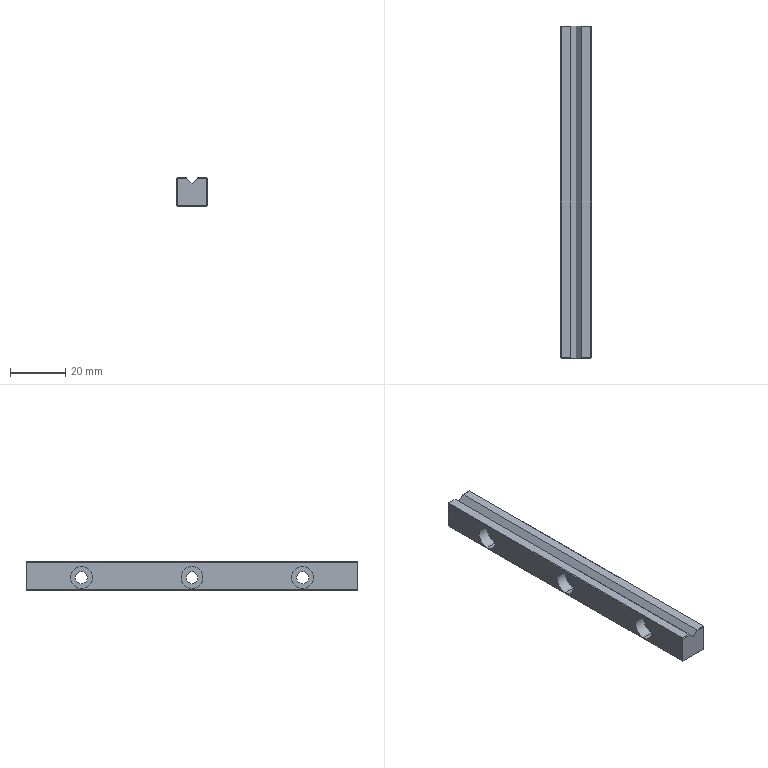Part | STEP file | 1 solid | 38 faces | box 11 x 120 x 10.2 mm | volume 12030 mm3 | plane 26 | cylinder 12 | commonest cylinder face diameters 4.3 x6 8 x6
STEP:
#1=CARTESIAN_POINT('',(-12.5,22.5,-37.85));
#2=VERTEX_POINT('',#1);
#3=CARTESIAN_POINT('',(-12.5,22.5,-42.15));
#4=VERTEX_POINT('',#3);
#5=CARTESIAN_POINT('',(-12.5,22.5,-40.));
#6=DIRECTION('',(1.,0.,0.));
#7=DIRECTION('',(0.,0.,1.));
#8=AXIS2_PLACEMENT_3D('',#5,#6,#7);
#9=CIRCLE('',#8,2.15);
#10=EDGE_CURVE('',#2,#4,#9,.T.);
#11=ORIENTED_EDGE('',*,*,#10,.T.);
#12=CARTESIAN_POINT('',(-19.3,22.5,-42.15));
#13=VERTEX_POINT('',#12);
#14=CARTESIAN_POINT('',(-12.5,22.5,-42.15));
#15=DIRECTION('',(-1.,0.,0.));
#16=VECTOR('',#15,1000.);
#17=LINE('',#14,#16);
#18=EDGE_CURVE('',#4,#13,#17,.T.);
#19=ORIENTED_EDGE('',*,*,#18,.T.);
#20=CARTESIAN_POINT('',(-19.3,22.5,-37.85));
#21=VERTEX_POINT('',#20);
#22=CARTESIAN_POINT('',(-19.3,22.5,-40.));
#23=DIRECTION('',(1.,0.,0.));
#24=DIRECTION('',(0.,0.,1.));
#25=AXIS2_PLACEMENT_3D('',#22,#23,#24);
#26=CIRCLE('',#25,2.15);
#27=EDGE_CURVE('',#21,#13,#26,.T.);
#28=ORIENTED_EDGE('',*,*,#27,.F.);
#29=CARTESIAN_POINT('',(-12.5,22.5,-37.85));
#30=DIRECTION('',(-1.,0.,0.));
#31=VECTOR('',#30,1000.);
#32=LINE('',#29,#31);
#33=EDGE_CURVE('',#2,#21,#32,.T.);
#34=ORIENTED_EDGE('',*,*,#33,.F.);
#35=EDGE_LOOP('',(#11,#19,#28,#34));
#36=FACE_OUTER_BOUND('',#35,.T.);
#37=CARTESIAN_POINT('',(-12.5,22.5,-40.));
#38=DIRECTION('',(-1.,0.,0.));
#39=DIRECTION('',(0.,0.,1.));
#40=AXIS2_PLACEMENT_3D('',#37,#38,#39);
#41=CYLINDRICAL_SURFACE('',#40,2.15);
#42=ADVANCED_FACE('',(#36),#41,.F.);
#43=CARTESIAN_POINT('',(-12.5,-17.5,-37.85));
#44=VERTEX_POINT('',#43);
#45=CARTESIAN_POINT('',(-12.5,-17.5,-42.15));
#46=VERTEX_POINT('',#45);
#47=CARTESIAN_POINT('',(-12.5,-17.5,-40.));
#48=DIRECTION('',(1.,0.,0.));
#49=DIRECTION('',(0.,0.,1.));
#50=AXIS2_PLACEMENT_3D('',#47,#48,#49);
#51=CIRCLE('',#50,2.15);
#52=EDGE_CURVE('',#44,#46,#51,.T.);
#53=ORIENTED_EDGE('',*,*,#52,.T.);
#54=CARTESIAN_POINT('',(-19.3,-17.5,-42.15));
#55=VERTEX_POINT('',#54);
#56=CARTESIAN_POINT('',(-12.5,-17.5,-42.15));
#57=DIRECTION('',(-1.,0.,0.));
#58=VECTOR('',#57,1000.);
#59=LINE('',#56,#58);
#60=EDGE_CURVE('',#46,#55,#59,.T.);
#61=ORIENTED_EDGE('',*,*,#60,.T.);
#62=CARTESIAN_POINT('',(-19.3,-17.5,-37.85));
#63=VERTEX_POINT('',#62);
#64=CARTESIAN_POINT('',(-19.3,-17.5,-40.));
#65=DIRECTION('',(1.,0.,0.));
#66=DIRECTION('',(0.,0.,1.));
#67=AXIS2_PLACEMENT_3D('',#64,#65,#66);
#68=CIRCLE('',#67,2.15);
#69=EDGE_CURVE('',#63,#55,#68,.T.);
#70=ORIENTED_EDGE('',*,*,#69,.F.);
#71=CARTESIAN_POINT('',(-12.5,-17.5,-37.85));
#72=DIRECTION('',(-1.,0.,0.));
#73=VECTOR('',#72,1000.);
#74=LINE('',#71,#73);
#75=EDGE_CURVE('',#44,#63,#74,.T.);
#76=ORIENTED_EDGE('',*,*,#75,.F.);
#77=EDGE_LOOP('',(#53,#61,#70,#76));
#78=FACE_OUTER_BOUND('',#77,.T.);
#79=CARTESIAN_POINT('',(-12.5,-17.5,-40.));
#80=DIRECTION('',(-1.,0.,0.));
#81=DIRECTION('',(0.,0.,1.));
#82=AXIS2_PLACEMENT_3D('',#79,#80,#81);
#83=CYLINDRICAL_SURFACE('',#82,2.15);
#84=ADVANCED_FACE('',(#78),#83,.F.);
#85=CARTESIAN_POINT('',(-12.5,-57.5,-37.85));
#86=VERTEX_POINT('',#85);
#87=CARTESIAN_POINT('',(-12.5,-57.5,-42.15));
#88=VERTEX_POINT('',#87);
#89=CARTESIAN_POINT('',(-12.5,-57.5,-40.));
#90=DIRECTION('',(1.,0.,0.));
#91=DIRECTION('',(0.,0.,1.));
#92=AXIS2_PLACEMENT_3D('',#89,#90,#91);
#93=CIRCLE('',#92,2.15);
#94=EDGE_CURVE('',#86,#88,#93,.T.);
#95=ORIENTED_EDGE('',*,*,#94,.T.);
#96=CARTESIAN_POINT('',(-19.3,-57.5,-42.15));
#97=VERTEX_POINT('',#96);
#98=CARTESIAN_POINT('',(-12.5,-57.5,-42.15));
#99=DIRECTION('',(-1.,0.,0.));
#100=VECTOR('',#99,1000.);
#101=LINE('',#98,#100);
#102=EDGE_CURVE('',#88,#97,#101,.T.);
#103=ORIENTED_EDGE('',*,*,#102,.T.);
#104=CARTESIAN_POINT('',(-19.3,-57.5,-37.85));
#105=VERTEX_POINT('',#104);
#106=CARTESIAN_POINT('',(-19.3,-57.5,-40.));
#107=DIRECTION('',(1.,0.,0.));
#108=DIRECTION('',(0.,0.,1.));
#109=AXIS2_PLACEMENT_3D('',#106,#107,#108);
#110=CIRCLE('',#109,2.15);
#111=EDGE_CURVE('',#105,#97,#110,.T.);
#112=ORIENTED_EDGE('',*,*,#111,.F.);
#113=CARTESIAN_POINT('',(-12.5,-57.5,-37.85));
#114=DIRECTION('',(-1.,0.,0.));
#115=VECTOR('',#114,1000.);
#116=LINE('',#113,#115);
#117=EDGE_CURVE('',#86,#105,#116,.T.);
#118=ORIENTED_EDGE('',*,*,#117,.F.);
#119=EDGE_LOOP('',(#95,#103,#112,#118));
#120=FACE_OUTER_BOUND('',#119,.T.);
#121=CARTESIAN_POINT('',(-12.5,-57.5,-40.));
#122=DIRECTION('',(-1.,0.,0.));
#123=DIRECTION('',(0.,0.,1.));
#124=AXIS2_PLACEMENT_3D('',#121,#122,#123);
#125=CYLINDRICAL_SURFACE('',#124,2.15);
#126=ADVANCED_FACE('',(#120),#125,.F.);
#127=CARTESIAN_POINT('',(-19.3,22.5,-44.));
#128=VERTEX_POINT('',#127);
#129=CARTESIAN_POINT('',(-19.3,22.5,-36.));
#130=VERTEX_POINT('',#129);
#131=CARTESIAN_POINT('',(-19.3,22.5,-40.));
#132=DIRECTION('',(-1.,0.,0.));
#133=DIRECTION('',(0.,0.,1.));
#134=AXIS2_PLACEMENT_3D('',#131,#132,#133);
#135=CIRCLE('',#134,4.);
#136=EDGE_CURVE('',#128,#130,#135,.T.);
#137=ORIENTED_EDGE('',*,*,#136,.F.);
#138=CARTESIAN_POINT('',(-23.5,22.5,-44.));
#139=VERTEX_POINT('',#138);
#140=CARTESIAN_POINT('',(-19.3,22.5,-44.));
#141=DIRECTION('',(-1.,0.,0.));
#142=VECTOR('',#141,1000.);
#143=LINE('',#140,#142);
#144=EDGE_CURVE('',#128,#139,#143,.T.);
#145=ORIENTED_EDGE('',*,*,#144,.T.);
#146=CARTESIAN_POINT('',(-23.5,22.5,-36.));
#147=VERTEX_POINT('',#146);
#148=CARTESIAN_POINT('',(-23.5,22.5,-40.));
#149=DIRECTION('',(-1.,0.,0.));
#150=DIRECTION('',(0.,0.,1.));
#151=AXIS2_PLACEMENT_3D('',#148,#149,#150);
#152=CIRCLE('',#151,4.);
#153=EDGE_CURVE('',#139,#147,#152,.T.);
#154=ORIENTED_EDGE('',*,*,#153,.T.);
#155=CARTESIAN_POINT('',(-19.3,22.5,-36.));
#156=DIRECTION('',(-1.,0.,0.));
#157=VECTOR('',#156,1000.);
#158=LINE('',#155,#157);
#159=EDGE_CURVE('',#130,#147,#158,.T.);
#160=ORIENTED_EDGE('',*,*,#159,.F.);
#161=EDGE_LOOP('',(#137,#145,#154,#160));
#162=FACE_OUTER_BOUND('',#161,.T.);
#163=CARTESIAN_POINT('',(-19.3,22.5,-40.));
#164=DIRECTION('',(-1.,0.,0.));
#165=DIRECTION('',(0.,0.,1.));
#166=AXIS2_PLACEMENT_3D('',#163,#164,#165);
#167=CYLINDRICAL_SURFACE('',#166,4.);
#168=ADVANCED_FACE('',(#162),#167,.F.);
#169=CARTESIAN_POINT('',(-19.3,-17.5,-44.));
#170=VERTEX_POINT('',#169);
#171=CARTESIAN_POINT('',(-19.3,-17.5,-36.));
#172=VERTEX_POINT('',#171);
#173=CARTESIAN_POINT('',(-19.3,-17.5,-40.));
#174=DIRECTION('',(-1.,0.,0.));
#175=DIRECTION('',(0.,0.,1.));
#176=AXIS2_PLACEMENT_3D('',#173,#174,#175);
#177=CIRCLE('',#176,4.);
#178=EDGE_CURVE('',#170,#172,#177,.T.);
#179=ORIENTED_EDGE('',*,*,#178,.F.);
#180=CARTESIAN_POINT('',(-23.5,-17.5,-44.));
#181=VERTEX_POINT('',#180);
#182=CARTESIAN_POINT('',(-19.3,-17.5,-44.));
#183=DIRECTION('',(-1.,0.,0.));
#184=VECTOR('',#183,1000.);
#185=LINE('',#182,#184);
#186=EDGE_CURVE('',#170,#181,#185,.T.);
#187=ORIENTED_EDGE('',*,*,#186,.T.);
#188=CARTESIAN_POINT('',(-23.5,-17.5,-36.));
#189=VERTEX_POINT('',#188);
#190=CARTESIAN_POINT('',(-23.5,-17.5,-40.));
#191=DIRECTION('',(-1.,0.,0.));
#192=DIRECTION('',(0.,0.,1.));
#193=AXIS2_PLACEMENT_3D('',#190,#191,#192);
#194=CIRCLE('',#193,4.);
#195=EDGE_CURVE('',#181,#189,#194,.T.);
#196=ORIENTED_EDGE('',*,*,#195,.T.);
#197=CARTESIAN_POINT('',(-19.3,-17.5,-36.));
#198=DIRECTION('',(-1.,0.,0.));
#199=VECTOR('',#198,1000.);
#200=LINE('',#197,#199);
#201=EDGE_CURVE('',#172,#189,#200,.T.);
#202=ORIENTED_EDGE('',*,*,#201,.F.);
#203=EDGE_LOOP('',(#179,#187,#196,#202));
#204=FACE_OUTER_BOUND('',#203,.T.);
#205=CARTESIAN_POINT('',(-19.3,-17.5,-40.));
#206=DIRECTION('',(-1.,0.,0.));
#207=DIRECTION('',(0.,0.,1.));
#208=AXIS2_PLACEMENT_3D('',#205,#206,#207);
#209=CYLINDRICAL_SURFACE('',#208,4.);
#210=ADVANCED_FACE('',(#204),#209,.F.);
#211=CARTESIAN_POINT('',(-19.3,-57.5,-44.));
#212=VERTEX_POINT('',#211);
#213=CARTESIAN_POINT('',(-19.3,-57.5,-36.));
#214=VERTEX_POINT('',#213);
#215=CARTESIAN_POINT('',(-19.3,-57.5,-40.));
#216=DIRECTION('',(-1.,0.,0.));
#217=DIRECTION('',(0.,0.,1.));
#218=AXIS2_PLACEMENT_3D('',#215,#216,#217);
#219=CIRCLE('',#218,4.);
#220=EDGE_CURVE('',#212,#214,#219,.T.);
#221=ORIENTED_EDGE('',*,*,#220,.F.);
#222=CARTESIAN_POINT('',(-23.5,-57.5,-44.));
#223=VERTEX_POINT('',#222);
#224=CARTESIAN_POINT('',(-19.3,-57.5,-44.));
#225=DIRECTION('',(-1.,0.,0.));
#226=VECTOR('',#225,1000.);
#227=LINE('',#224,#226);
#228=EDGE_CURVE('',#212,#223,#227,.T.);
#229=ORIENTED_EDGE('',*,*,#228,.T.);
#230=CARTESIAN_POINT('',(-23.5,-57.5,-36.));
#231=VERTEX_POINT('',#230);
#232=CARTESIAN_POINT('',(-23.5,-57.5,-40.));
#233=DIRECTION('',(-1.,0.,0.));
#234=DIRECTION('',(0.,0.,1.));
#235=AXIS2_PLACEMENT_3D('',#232,#233,#234);
#236=CIRCLE('',#235,4.);
#237=EDGE_CURVE('',#223,#231,#236,.T.);
#238=ORIENTED_EDGE('',*,*,#237,.T.);
#239=CARTESIAN_POINT('',(-19.3,-57.5,-36.));
#240=DIRECTION('',(-1.,0.,0.));
#241=VECTOR('',#240,1000.);
#242=LINE('',#239,#241);
#243=EDGE_CURVE('',#214,#231,#242,.T.);
#244=ORIENTED_EDGE('',*,*,#243,.F.);
#245=EDGE_LOOP('',(#221,#229,#238,#244));
#246=FACE_OUTER_BOUND('',#245,.T.);
#247=CARTESIAN_POINT('',(-19.3,-57.5,-40.));
#248=DIRECTION('',(-1.,0.,0.));
#249=DIRECTION('',(0.,0.,1.));
#250=AXIS2_PLACEMENT_3D('',#247,#248,#249);
#251=CYLINDRICAL_SURFACE('',#250,4.);
#252=ADVANCED_FACE('',(#246),#251,.F.);
#253=CARTESIAN_POINT('',(-16.172,42.5,-34.5));
#254=VERTEX_POINT('',#253);
#255=CARTESIAN_POINT('',(-18.,42.5,-36.328));
#256=VERTEX_POINT('',#255);
#257=CARTESIAN_POINT('',(-18.103,42.5,-36.431));
#258=DIRECTION('',(-0.7071,0.,-0.7071));
#259=VECTOR('',#258,1000.);
#260=LINE('',#257,#259);
#261=EDGE_CURVE('',#254,#256,#260,.T.);
#262=ORIENTED_EDGE('',*,*,#261,.F.);
#263=CARTESIAN_POINT('',(-12.7,42.5,-34.5));
#264=VERTEX_POINT('',#263);
#265=CARTESIAN_POINT('',(-18.,42.5,-34.5));
#266=DIRECTION('',(-1.,0.,0.));
#267=VECTOR('',#266,1000.);
#268=LINE('',#265,#267);
#269=EDGE_CURVE('',#264,#254,#268,.T.);
#270=ORIENTED_EDGE('',*,*,#269,.F.);
#271=CARTESIAN_POINT('',(-12.7,42.5,-44.3));
#272=VERTEX_POINT('',#271);
#273=CARTESIAN_POINT('',(-12.7,42.5,-39.4));
#274=DIRECTION('',(0.,0.,1.));
#275=VECTOR('',#274,1000.);
#276=LINE('',#273,#275);
#277=EDGE_CURVE('',#272,#264,#276,.T.);
#278=ORIENTED_EDGE('',*,*,#277,.F.);
#279=CARTESIAN_POINT('',(-23.3,42.5,-44.3));
#280=VERTEX_POINT('',#279);
#281=CARTESIAN_POINT('',(-18.,42.5,-44.3));
#282=DIRECTION('',(1.,0.,0.));
#283=VECTOR('',#282,1000.);
#284=LINE('',#281,#283);
#285=EDGE_CURVE('',#280,#272,#284,.T.);
#286=ORIENTED_EDGE('',*,*,#285,.F.);
#287=CARTESIAN_POINT('',(-23.3,42.5,-34.5));
#288=VERTEX_POINT('',#287);
#289=CARTESIAN_POINT('',(-23.3,42.5,-39.4));
#290=DIRECTION('',(0.,0.,-1.));
#291=VECTOR('',#290,1000.);
#292=LINE('',#289,#291);
#293=EDGE_CURVE('',#288,#280,#292,.T.);
#294=ORIENTED_EDGE('',*,*,#293,.F.);
#295=CARTESIAN_POINT('',(-19.828,42.5,-34.5));
#296=VERTEX_POINT('',#295);
#297=CARTESIAN_POINT('',(-18.,42.5,-34.5));
#298=DIRECTION('',(-1.,0.,0.));
#299=VECTOR('',#298,1000.);
#300=LINE('',#297,#299);
#301=EDGE_CURVE('',#296,#288,#300,.T.);
#302=ORIENTED_EDGE('',*,*,#301,.F.);
#303=CARTESIAN_POINT('',(-20.131,42.5,-34.197));
#304=DIRECTION('',(-0.7071,0.,0.7071));
#305=VECTOR('',#304,1000.);
#306=LINE('',#303,#305);
#307=EDGE_CURVE('',#256,#296,#306,.T.);
#308=ORIENTED_EDGE('',*,*,#307,.F.);
#309=EDGE_LOOP('',(#262,#270,#278,#286,#294,#302,#308));
#310=FACE_OUTER_BOUND('',#309,.T.);
#311=CARTESIAN_POINT('',(-12.488,42.5,-34.304));
#312=DIRECTION('',(0.,-1.,0.));
#313=DIRECTION('',(-1.,0.,0.));
#314=AXIS2_PLACEMENT_3D('',#311,#312,#313);
#315=PLANE('',#314);
#316=ADVANCED_FACE('',(#310),#315,.F.);
#317=CARTESIAN_POINT('',(-18.,-77.5,-36.328));
#318=VERTEX_POINT('',#317);
#319=CARTESIAN_POINT('',(-18.,-17.5,-36.328));
#320=DIRECTION('',(0.,-1.,0.));
#321=VECTOR('',#320,1000.);
#322=LINE('',#319,#321);
#323=EDGE_CURVE('',#256,#318,#322,.T.);
#324=ORIENTED_EDGE('',*,*,#323,.F.);
#325=ORIENTED_EDGE('',*,*,#307,.T.);
#326=CARTESIAN_POINT('',(-20.028,42.3,-34.3));
#327=VERTEX_POINT('',#326);
#328=CARTESIAN_POINT('',(-20.028,42.3,-34.3));
#329=DIRECTION('',(0.5774,0.5774,-0.5774));
#330=VECTOR('',#329,1000.);
#331=LINE('',#328,#330);
#332=EDGE_CURVE('',#327,#296,#331,.T.);
#333=ORIENTED_EDGE('',*,*,#332,.F.);
#334=CARTESIAN_POINT('',(-20.028,-77.3,-34.3));
#335=VERTEX_POINT('',#334);
#336=CARTESIAN_POINT('',(-20.028,-17.5,-34.3));
#337=DIRECTION('',(0.,1.,0.));
#338=VECTOR('',#337,1000.);
#339=LINE('',#336,#338);
#340=EDGE_CURVE('',#335,#327,#339,.T.);
#341=ORIENTED_EDGE('',*,*,#340,.F.);
#342=CARTESIAN_POINT('',(-19.828,-77.5,-34.5));
#343=VERTEX_POINT('',#342);
#344=CARTESIAN_POINT('',(-20.028,-77.3,-34.3));
#345=DIRECTION('',(0.5774,-0.5774,-0.5774));
#346=VECTOR('',#345,1000.);
#347=LINE('',#344,#346);
#348=EDGE_CURVE('',#335,#343,#347,.T.);
#349=ORIENTED_EDGE('',*,*,#348,.T.);
#350=CARTESIAN_POINT('',(-19.014,-77.5,-35.314));
#351=DIRECTION('',(-0.7071,0.,0.7071));
#352=VECTOR('',#351,1000.);
#353=LINE('',#350,#352);
#354=EDGE_CURVE('',#318,#343,#353,.T.);
#355=ORIENTED_EDGE('',*,*,#354,.F.);
#356=EDGE_LOOP('',(#324,#325,#333,#341,#349,#355));
#357=FACE_OUTER_BOUND('',#356,.T.);
#358=CARTESIAN_POINT('',(-20.131,44.9,-34.197));
#359=DIRECTION('',(-0.7071,0.,-0.7071));
#360=DIRECTION('',(0.7071,0.,-0.7071));
#361=AXIS2_PLACEMENT_3D('',#358,#359,#360);
#362=PLANE('',#361);
#363=ADVANCED_FACE('',(#357),#362,.F.);
#364=CARTESIAN_POINT('',(-15.972,42.3,-34.3));
#365=VERTEX_POINT('',#364);
#366=CARTESIAN_POINT('',(-16.172,42.5,-34.5));
#367=DIRECTION('',(0.5774,-0.5774,0.5774));
#368=VECTOR('',#367,1000.);
#369=LINE('',#366,#368);
#370=EDGE_CURVE('',#254,#365,#369,.T.);
#371=ORIENTED_EDGE('',*,*,#370,.F.);
#372=ORIENTED_EDGE('',*,*,#261,.T.);
#373=ORIENTED_EDGE('',*,*,#323,.T.);
#374=CARTESIAN_POINT('',(-16.172,-77.5,-34.5));
#375=VERTEX_POINT('',#374);
#376=CARTESIAN_POINT('',(-16.986,-77.5,-35.314));
#377=DIRECTION('',(-0.7071,0.,-0.7071));
#378=VECTOR('',#377,1000.);
#379=LINE('',#376,#378);
#380=EDGE_CURVE('',#375,#318,#379,.T.);
#381=ORIENTED_EDGE('',*,*,#380,.F.);
#382=CARTESIAN_POINT('',(-15.972,-77.3,-34.3));
#383=VERTEX_POINT('',#382);
#384=CARTESIAN_POINT('',(-16.172,-77.5,-34.5));
#385=DIRECTION('',(0.5774,0.5774,0.5774));
#386=VECTOR('',#385,1000.);
#387=LINE('',#384,#386);
#388=EDGE_CURVE('',#375,#383,#387,.T.);
#389=ORIENTED_EDGE('',*,*,#388,.T.);
#390=CARTESIAN_POINT('',(-15.972,-17.5,-34.3));
#391=DIRECTION('',(0.,-1.,0.));
#392=VECTOR('',#391,1000.);
#393=LINE('',#390,#392);
#394=EDGE_CURVE('',#365,#383,#393,.T.);
#395=ORIENTED_EDGE('',*,*,#394,.F.);
#396=EDGE_LOOP('',(#371,#372,#373,#381,#389,#395));
#397=FACE_OUTER_BOUND('',#396,.T.);
#398=CARTESIAN_POINT('',(-18.103,44.9,-36.431));
#399=DIRECTION('',(0.7071,0.,-0.7071));
#400=DIRECTION('',(0.7071,0.,0.7071));
#401=AXIS2_PLACEMENT_3D('',#398,#399,#400);
#402=PLANE('',#401);
#403=ADVANCED_FACE('',(#397),#402,.F.);
#404=CARTESIAN_POINT('',(-12.7,42.3,-34.3));
#405=VERTEX_POINT('',#404);
#406=CARTESIAN_POINT('',(-12.6,42.4,-34.4));
#407=VERTEX_POINT('',#406);
#408=CARTESIAN_POINT('',(-12.7,42.3,-34.3));
#409=DIRECTION('',(0.5774,0.5774,-0.5774));
#410=VECTOR('',#409,1000.);
#411=LINE('',#408,#410);
#412=EDGE_CURVE('',#405,#407,#411,.T.);
#413=ORIENTED_EDGE('',*,*,#412,.T.);
#414=CARTESIAN_POINT('',(-12.7,42.5,-34.5));
#415=DIRECTION('',(0.5774,-0.5774,0.5774));
#416=VECTOR('',#415,1000.);
#417=LINE('',#414,#416);
#418=EDGE_CURVE('',#264,#407,#417,.T.);
#419=ORIENTED_EDGE('',*,*,#418,.F.);
#420=ORIENTED_EDGE('',*,*,#269,.T.);
#421=ORIENTED_EDGE('',*,*,#370,.T.);
#422=CARTESIAN_POINT('',(-14.386,42.3,-34.3));
#423=DIRECTION('',(-1.,0.,0.));
#424=VECTOR('',#423,1000.);
#425=LINE('',#422,#424);
#426=EDGE_CURVE('',#405,#365,#425,.T.);
#427=ORIENTED_EDGE('',*,*,#426,.F.);
#428=EDGE_LOOP('',(#413,#419,#420,#421,#427));
#429=FACE_OUTER_BOUND('',#428,.T.);
#430=CARTESIAN_POINT('',(-16.317,42.603,-34.603));
#431=DIRECTION('',(0.,0.7071,0.7071));
#432=DIRECTION('',(0.,-0.7071,0.7071));
#433=AXIS2_PLACEMENT_3D('',#430,#431,#432);
#434=PLANE('',#433);
#435=ADVANCED_FACE('',(#429),#434,.T.);
#436=CARTESIAN_POINT('',(-12.6,42.4,-44.4));
#437=VERTEX_POINT('',#436);
#438=CARTESIAN_POINT('',(-12.7,42.5,-44.3));
#439=DIRECTION('',(0.5774,-0.5774,-0.5774));
#440=VECTOR('',#439,1000.);
#441=LINE('',#438,#440);
#442=EDGE_CURVE('',#272,#437,#441,.T.);
#443=ORIENTED_EDGE('',*,*,#442,.F.);
#444=ORIENTED_EDGE('',*,*,#277,.T.);
#445=ORIENTED_EDGE('',*,*,#418,.T.);
#446=CARTESIAN_POINT('',(-12.5,42.3,-34.5));
#447=VERTEX_POINT('',#446);
#448=CARTESIAN_POINT('',(-12.6,42.4,-34.4));
#449=DIRECTION('',(0.5774,-0.5774,-0.5774));
#450=VECTOR('',#449,1000.);
#451=LINE('',#448,#450);
#452=EDGE_CURVE('',#407,#447,#451,.T.);
#453=ORIENTED_EDGE('',*,*,#452,.T.);
#454=CARTESIAN_POINT('',(-12.5,42.3,-44.3));
#455=VERTEX_POINT('',#454);
#456=CARTESIAN_POINT('',(-12.5,42.3,-39.4));
#457=DIRECTION('',(0.,0.,1.));
#458=VECTOR('',#457,1000.);
#459=LINE('',#456,#458);
#460=EDGE_CURVE('',#455,#447,#459,.T.);
#461=ORIENTED_EDGE('',*,*,#460,.F.);
#462=CARTESIAN_POINT('',(-12.5,42.3,-44.3));
#463=DIRECTION('',(-0.5774,0.5774,-0.5774));
#464=VECTOR('',#463,1000.);
#465=LINE('',#462,#464);
#466=EDGE_CURVE('',#455,#437,#465,.T.);
#467=ORIENTED_EDGE('',*,*,#466,.T.);
#468=EDGE_LOOP('',(#443,#444,#445,#453,#461,#467));
#469=FACE_OUTER_BOUND('',#468,.T.);
#470=CARTESIAN_POINT('',(-12.803,42.603,-34.2));
#471=DIRECTION('',(0.7071,0.7071,0.));
#472=DIRECTION('',(0.7071,-0.7071,0.));
#473=AXIS2_PLACEMENT_3D('',#470,#471,#472);
#474=PLANE('',#473);
#475=ADVANCED_FACE('',(#469),#474,.T.);
#476=CARTESIAN_POINT('',(-23.4,42.4,-44.4));
#477=VERTEX_POINT('',#476);
#478=CARTESIAN_POINT('',(-23.3,42.5,-44.3));
#479=DIRECTION('',(-0.5774,-0.5774,-0.5774));
#480=VECTOR('',#479,1000.);
#481=LINE('',#478,#480);
#482=EDGE_CURVE('',#280,#477,#481,.T.);
#483=ORIENTED_EDGE('',*,*,#482,.F.);
#484=ORIENTED_EDGE('',*,*,#285,.T.);
#485=ORIENTED_EDGE('',*,*,#442,.T.);
#486=CARTESIAN_POINT('',(-12.7,42.3,-44.5));
#487=VERTEX_POINT('',#486);
#488=CARTESIAN_POINT('',(-12.6,42.4,-44.4));
#489=DIRECTION('',(-0.5774,-0.5774,-0.5774));
#490=VECTOR('',#489,1000.);
#491=LINE('',#488,#490);
#492=EDGE_CURVE('',#437,#487,#491,.T.);
#493=ORIENTED_EDGE('',*,*,#492,.T.);
#494=CARTESIAN_POINT('',(-23.3,42.3,-44.5));
#495=VERTEX_POINT('',#494);
#496=CARTESIAN_POINT('',(-18.,42.3,-44.5));
#497=DIRECTION('',(1.,0.,0.));
#498=VECTOR('',#497,1000.);
#499=LINE('',#496,#498);
#500=EDGE_CURVE('',#495,#487,#499,.T.);
#501=ORIENTED_EDGE('',*,*,#500,.F.);
#502=CARTESIAN_POINT('',(-23.3,42.3,-44.5));
#503=DIRECTION('',(-0.5774,0.5774,0.5774));
#504=VECTOR('',#503,1000.);
#505=LINE('',#502,#504);
#506=EDGE_CURVE('',#495,#477,#505,.T.);
#507=ORIENTED_EDGE('',*,*,#506,.T.);
#508=EDGE_LOOP('',(#483,#484,#485,#493,#501,#507));
#509=FACE_OUTER_BOUND('',#508,.T.);
#510=CARTESIAN_POINT('',(-12.384,42.603,-44.197));
#511=DIRECTION('',(0.,0.7071,-0.7071));
#512=DIRECTION('',(0.,-0.7071,-0.7071));
#513=AXIS2_PLACEMENT_3D('',#510,#511,#512);
#514=PLANE('',#513);
#515=ADVANCED_FACE('',(#509),#514,.T.);
#516=CARTESIAN_POINT('',(-23.5,42.3,-44.3));
#517=VERTEX_POINT('',#516);
#518=CARTESIAN_POINT('',(-23.4,42.4,-44.4));
#519=DIRECTION('',(-0.5774,-0.5774,0.5774));
#520=VECTOR('',#519,1000.);
#521=LINE('',#518,#520);
#522=EDGE_CURVE('',#477,#517,#521,.T.);
#523=ORIENTED_EDGE('',*,*,#522,.T.);
#524=CARTESIAN_POINT('',(-23.5,42.3,-34.5));
#525=VERTEX_POINT('',#524);
#526=CARTESIAN_POINT('',(-23.5,42.3,-39.4));
#527=DIRECTION('',(0.,0.,-1.));
#528=VECTOR('',#527,1000.);
#529=LINE('',#526,#528);
#530=EDGE_CURVE('',#525,#517,#529,.T.);
#531=ORIENTED_EDGE('',*,*,#530,.F.);
#532=CARTESIAN_POINT('',(-23.4,42.4,-34.4));
#533=VERTEX_POINT('',#532);
#534=CARTESIAN_POINT('',(-23.5,42.3,-34.5));
#535=DIRECTION('',(0.5774,0.5774,0.5774));
#536=VECTOR('',#535,1000.);
#537=LINE('',#534,#536);
#538=EDGE_CURVE('',#525,#533,#537,.T.);
#539=ORIENTED_EDGE('',*,*,#538,.T.);
#540=CARTESIAN_POINT('',(-23.3,42.5,-34.5));
#541=DIRECTION('',(-0.5774,-0.5774,0.5774));
#542=VECTOR('',#541,1000.);
#543=LINE('',#540,#542);
#544=EDGE_CURVE('',#288,#533,#543,.T.);
#545=ORIENTED_EDGE('',*,*,#544,.F.);
#546=ORIENTED_EDGE('',*,*,#293,.T.);
#547=ORIENTED_EDGE('',*,*,#482,.T.);
#548=EDGE_LOOP('',(#523,#531,#539,#545,#546,#547));
#549=FACE_OUTER_BOUND('',#548,.T.);
#550=CARTESIAN_POINT('',(-23.197,42.603,-44.6));
#551=DIRECTION('',(-0.7071,0.7071,0.));
#552=DIRECTION('',(-0.7071,-0.7071,0.));
#553=AXIS2_PLACEMENT_3D('',#550,#551,#552);
#554=PLANE('',#553);
#555=ADVANCED_FACE('',(#549),#554,.T.);
#556=ORIENTED_EDGE('',*,*,#544,.T.);
#557=CARTESIAN_POINT('',(-23.3,42.3,-34.3));
#558=VERTEX_POINT('',#557);
#559=CARTESIAN_POINT('',(-23.4,42.4,-34.4));
#560=DIRECTION('',(0.5774,-0.5774,0.5774));
#561=VECTOR('',#560,1000.);
#562=LINE('',#559,#561);
#563=EDGE_CURVE('',#533,#558,#562,.T.);
#564=ORIENTED_EDGE('',*,*,#563,.T.);
#565=CARTESIAN_POINT('',(-21.614,42.3,-34.3));
#566=DIRECTION('',(-1.,0.,0.));
#567=VECTOR('',#566,1000.);
#568=LINE('',#565,#567);
#569=EDGE_CURVE('',#327,#558,#568,.T.);
#570=ORIENTED_EDGE('',*,*,#569,.F.);
#571=ORIENTED_EDGE('',*,*,#332,.T.);
#572=ORIENTED_EDGE('',*,*,#301,.T.);
#573=EDGE_LOOP('',(#556,#564,#570,#571,#572));
#574=FACE_OUTER_BOUND('',#573,.T.);
#575=CARTESIAN_POINT('',(-23.545,42.603,-34.603));
#576=DIRECTION('',(0.,0.7071,0.7071));
#577=DIRECTION('',(0.,-0.7071,0.7071));
#578=AXIS2_PLACEMENT_3D('',#575,#576,#577);
#579=PLANE('',#578);
#580=ADVANCED_FACE('',(#574),#579,.T.);
#581=CARTESIAN_POINT('',(-12.7,-77.5,-44.3));
#582=VERTEX_POINT('',#581);
#583=CARTESIAN_POINT('',(-23.3,-77.5,-44.3));
#584=VERTEX_POINT('',#583);
#585=CARTESIAN_POINT('',(-18.,-77.5,-44.3));
#586=DIRECTION('',(-1.,0.,0.));
#587=VECTOR('',#586,1000.);
#588=LINE('',#585,#587);
#589=EDGE_CURVE('',#582,#584,#588,.T.);
#590=ORIENTED_EDGE('',*,*,#589,.F.);
#591=CARTESIAN_POINT('',(-12.7,-77.5,-34.5));
#592=VERTEX_POINT('',#591);
#593=CARTESIAN_POINT('',(-12.7,-77.5,-39.4));
#594=DIRECTION('',(0.,0.,-1.));
#595=VECTOR('',#594,1000.);
#596=LINE('',#593,#595);
#597=EDGE_CURVE('',#592,#582,#596,.T.);
#598=ORIENTED_EDGE('',*,*,#597,.F.);
#599=CARTESIAN_POINT('',(-18.,-77.5,-34.5));
#600=DIRECTION('',(1.,0.,0.));
#601=VECTOR('',#600,1000.);
#602=LINE('',#599,#601);
#603=EDGE_CURVE('',#375,#592,#602,.T.);
#604=ORIENTED_EDGE('',*,*,#603,.F.);
#605=ORIENTED_EDGE('',*,*,#380,.T.);
#606=ORIENTED_EDGE('',*,*,#354,.T.);
#607=CARTESIAN_POINT('',(-23.3,-77.5,-34.5));
#608=VERTEX_POINT('',#607);
#609=CARTESIAN_POINT('',(-18.,-77.5,-34.5));
#610=DIRECTION('',(1.,0.,0.));
#611=VECTOR('',#610,1000.);
#612=LINE('',#609,#611);
#613=EDGE_CURVE('',#608,#343,#612,.T.);
#614=ORIENTED_EDGE('',*,*,#613,.F.);
#615=CARTESIAN_POINT('',(-23.3,-77.5,-39.4));
#616=DIRECTION('',(0.,0.,1.));
#617=VECTOR('',#616,1000.);
#618=LINE('',#615,#617);
#619=EDGE_CURVE('',#584,#608,#618,.T.);
#620=ORIENTED_EDGE('',*,*,#619,.F.);
#621=EDGE_LOOP('',(#590,#598,#604,#605,#606,#614,#620));
#622=FACE_OUTER_BOUND('',#621,.T.);
#623=CARTESIAN_POINT('',(-12.488,-77.5,-34.304));
#624=DIRECTION('',(0.,-1.,0.));
#625=DIRECTION('',(-1.,0.,0.));
#626=AXIS2_PLACEMENT_3D('',#623,#624,#625);
#627=PLANE('',#626);
#628=ADVANCED_FACE('',(#622),#627,.T.);
#629=ORIENTED_EDGE('',*,*,#569,.T.);
#630=CARTESIAN_POINT('',(-23.3,-77.3,-34.3));
#631=VERTEX_POINT('',#630);
#632=CARTESIAN_POINT('',(-23.3,-17.5,-34.3));
#633=DIRECTION('',(0.,1.,0.));
#634=VECTOR('',#633,1000.);
#635=LINE('',#632,#634);
#636=EDGE_CURVE('',#631,#558,#635,.T.);
#637=ORIENTED_EDGE('',*,*,#636,.F.);
#638=CARTESIAN_POINT('',(-21.664,-77.3,-34.3));
#639=DIRECTION('',(-1.,0.,0.));
#640=VECTOR('',#639,1000.);
#641=LINE('',#638,#640);
#642=EDGE_CURVE('',#335,#631,#641,.T.);
#643=ORIENTED_EDGE('',*,*,#642,.F.);
#644=ORIENTED_EDGE('',*,*,#340,.T.);
#645=EDGE_LOOP('',(#629,#637,#643,#644));
#646=FACE_OUTER_BOUND('',#645,.T.);
#647=CARTESIAN_POINT('',(-19.883,44.692,-34.3));
#648=DIRECTION('',(0.,0.,1.));
#649=DIRECTION('',(-1.,0.,0.));
#650=AXIS2_PLACEMENT_3D('',#647,#648,#649);
#651=PLANE('',#650);
#652=ADVANCED_FACE('',(#646),#651,.T.);
#653=ORIENTED_EDGE('',*,*,#426,.T.);
#654=ORIENTED_EDGE('',*,*,#394,.T.);
#655=CARTESIAN_POINT('',(-12.7,-77.3,-34.3));
#656=VERTEX_POINT('',#655);
#657=CARTESIAN_POINT('',(-14.336,-77.3,-34.3));
#658=DIRECTION('',(-1.,0.,0.));
#659=VECTOR('',#658,1000.);
#660=LINE('',#657,#659);
#661=EDGE_CURVE('',#656,#383,#660,.T.);
#662=ORIENTED_EDGE('',*,*,#661,.F.);
#663=CARTESIAN_POINT('',(-12.7,-17.5,-34.3));
#664=DIRECTION('',(0.,-1.,0.));
#665=VECTOR('',#664,1000.);
#666=LINE('',#663,#665);
#667=EDGE_CURVE('',#405,#656,#666,.T.);
#668=ORIENTED_EDGE('',*,*,#667,.F.);
#669=EDGE_LOOP('',(#653,#654,#662,#668));
#670=FACE_OUTER_BOUND('',#669,.T.);
#671=CARTESIAN_POINT('',(-12.555,44.692,-34.3));
#672=DIRECTION('',(0.,0.,1.));
#673=DIRECTION('',(-1.,0.,0.));
#674=AXIS2_PLACEMENT_3D('',#671,#672,#673);
#675=PLANE('',#674);
#676=ADVANCED_FACE('',(#670),#675,.T.);
#677=ORIENTED_EDGE('',*,*,#10,.F.);
#678=CARTESIAN_POINT('',(-12.5,22.5,-40.));
#679=DIRECTION('',(1.,0.,0.));
#680=DIRECTION('',(0.,0.,1.));
#681=AXIS2_PLACEMENT_3D('',#678,#679,#680);
#682=CIRCLE('',#681,2.15);
#683=EDGE_CURVE('',#4,#2,#682,.T.);
#684=ORIENTED_EDGE('',*,*,#683,.F.);
#685=EDGE_LOOP('',(#677,#684));
#686=FACE_BOUND('',#685,.T.);
#687=ORIENTED_EDGE('',*,*,#52,.F.);
#688=CARTESIAN_POINT('',(-12.5,-17.5,-40.));
#689=DIRECTION('',(1.,0.,0.));
#690=DIRECTION('',(0.,0.,1.));
#691=AXIS2_PLACEMENT_3D('',#688,#689,#690);
#692=CIRCLE('',#691,2.15);
#693=EDGE_CURVE('',#46,#44,#692,.T.);
#694=ORIENTED_EDGE('',*,*,#693,.F.);
#695=EDGE_LOOP('',(#687,#694));
#696=FACE_BOUND('',#695,.T.);
#697=ORIENTED_EDGE('',*,*,#94,.F.);
#698=CARTESIAN_POINT('',(-12.5,-57.5,-40.));
#699=DIRECTION('',(1.,0.,0.));
#700=DIRECTION('',(0.,0.,1.));
#701=AXIS2_PLACEMENT_3D('',#698,#699,#700);
#702=CIRCLE('',#701,2.15);
#703=EDGE_CURVE('',#88,#86,#702,.T.);
#704=ORIENTED_EDGE('',*,*,#703,.F.);
#705=EDGE_LOOP('',(#697,#704));
#706=FACE_BOUND('',#705,.T.);
#707=CARTESIAN_POINT('',(-12.5,-77.3,-44.3));
#708=VERTEX_POINT('',#707);
#709=CARTESIAN_POINT('',(-12.5,-77.3,-34.5));
#710=VERTEX_POINT('',#709);
#711=CARTESIAN_POINT('',(-12.5,-77.3,-39.4));
#712=DIRECTION('',(0.,0.,1.));
#713=VECTOR('',#712,1000.);
#714=LINE('',#711,#713);
#715=EDGE_CURVE('',#708,#710,#714,.T.);
#716=ORIENTED_EDGE('',*,*,#715,.F.);
#717=CARTESIAN_POINT('',(-12.5,-17.5,-44.3));
#718=DIRECTION('',(0.,-1.,0.));
#719=VECTOR('',#718,1000.);
#720=LINE('',#717,#719);
#721=EDGE_CURVE('',#455,#708,#720,.T.);
#722=ORIENTED_EDGE('',*,*,#721,.F.);
#723=ORIENTED_EDGE('',*,*,#460,.T.);
#724=CARTESIAN_POINT('',(-12.5,-17.5,-34.5));
#725=DIRECTION('',(0.,1.,0.));
#726=VECTOR('',#725,1000.);
#727=LINE('',#724,#726);
#728=EDGE_CURVE('',#710,#447,#727,.T.);
#729=ORIENTED_EDGE('',*,*,#728,.F.);
#730=EDGE_LOOP('',(#716,#722,#723,#729));
#731=FACE_OUTER_BOUND('',#730,.T.);
#732=CARTESIAN_POINT('',(-12.5,44.692,-44.496));
#733=DIRECTION('',(1.,0.,0.));
#734=DIRECTION('',(0.,0.,1.));
#735=AXIS2_PLACEMENT_3D('',#732,#733,#734);
#736=PLANE('',#735);
#737=ADVANCED_FACE('',(#686,#696,#706,#731),#736,.T.);
#738=ORIENTED_EDGE('',*,*,#500,.T.);
#739=CARTESIAN_POINT('',(-12.7,-77.3,-44.5));
#740=VERTEX_POINT('',#739);
#741=CARTESIAN_POINT('',(-12.7,-17.5,-44.5));
#742=DIRECTION('',(0.,1.,0.));
#743=VECTOR('',#742,1000.);
#744=LINE('',#741,#743);
#745=EDGE_CURVE('',#740,#487,#744,.T.);
#746=ORIENTED_EDGE('',*,*,#745,.F.);
#747=CARTESIAN_POINT('',(-23.3,-77.3,-44.5));
#748=VERTEX_POINT('',#747);
#749=CARTESIAN_POINT('',(-18.,-77.3,-44.5));
#750=DIRECTION('',(1.,0.,0.));
#751=VECTOR('',#750,1000.);
#752=LINE('',#749,#751);
#753=EDGE_CURVE('',#748,#740,#752,.T.);
#754=ORIENTED_EDGE('',*,*,#753,.F.);
#755=CARTESIAN_POINT('',(-23.3,-17.5,-44.5));
#756=DIRECTION('',(0.,-1.,0.));
#757=VECTOR('',#756,1000.);
#758=LINE('',#755,#757);
#759=EDGE_CURVE('',#495,#748,#758,.T.);
#760=ORIENTED_EDGE('',*,*,#759,.F.);
#761=EDGE_LOOP('',(#738,#746,#754,#760));
#762=FACE_OUTER_BOUND('',#761,.T.);
#763=CARTESIAN_POINT('',(-23.512,44.692,-44.5));
#764=DIRECTION('',(0.,0.,-1.));
#765=DIRECTION('',(1.,0.,0.));
#766=AXIS2_PLACEMENT_3D('',#763,#764,#765);
#767=PLANE('',#766);
#768=ADVANCED_FACE('',(#762),#767,.T.);
#769=CARTESIAN_POINT('',(-23.5,22.5,-40.));
#770=DIRECTION('',(-1.,0.,0.));
#771=DIRECTION('',(0.,0.,1.));
#772=AXIS2_PLACEMENT_3D('',#769,#770,#771);
#773=CIRCLE('',#772,4.);
#774=EDGE_CURVE('',#147,#139,#773,.T.);
#775=ORIENTED_EDGE('',*,*,#774,.F.);
#776=ORIENTED_EDGE('',*,*,#153,.F.);
#777=EDGE_LOOP('',(#775,#776));
#778=FACE_BOUND('',#777,.T.);
#779=CARTESIAN_POINT('',(-23.5,-17.5,-40.));
#780=DIRECTION('',(-1.,0.,0.));
#781=DIRECTION('',(0.,0.,1.));
#782=AXIS2_PLACEMENT_3D('',#779,#780,#781);
#783=CIRCLE('',#782,4.);
#784=EDGE_CURVE('',#189,#181,#783,.T.);
#785=ORIENTED_EDGE('',*,*,#784,.F.);
#786=ORIENTED_EDGE('',*,*,#195,.F.);
#787=EDGE_LOOP('',(#785,#786));
#788=FACE_BOUND('',#787,.T.);
#789=CARTESIAN_POINT('',(-23.5,-57.5,-40.));
#790=DIRECTION('',(-1.,0.,0.));
#791=DIRECTION('',(0.,0.,1.));
#792=AXIS2_PLACEMENT_3D('',#789,#790,#791);
#793=CIRCLE('',#792,4.);
#794=EDGE_CURVE('',#231,#223,#793,.T.);
#795=ORIENTED_EDGE('',*,*,#794,.F.);
#796=ORIENTED_EDGE('',*,*,#237,.F.);
#797=EDGE_LOOP('',(#795,#796));
#798=FACE_BOUND('',#797,.T.);
#799=CARTESIAN_POINT('',(-23.5,-77.3,-34.5));
#800=VERTEX_POINT('',#799);
#801=CARTESIAN_POINT('',(-23.5,-77.3,-44.3));
#802=VERTEX_POINT('',#801);
#803=CARTESIAN_POINT('',(-23.5,-77.3,-39.4));
#804=DIRECTION('',(0.,0.,-1.));
#805=VECTOR('',#804,1000.);
#806=LINE('',#803,#805);
#807=EDGE_CURVE('',#800,#802,#806,.T.);
#808=ORIENTED_EDGE('',*,*,#807,.F.);
#809=CARTESIAN_POINT('',(-23.5,-17.5,-34.5));
#810=DIRECTION('',(0.,-1.,0.));
#811=VECTOR('',#810,1000.);
#812=LINE('',#809,#811);
#813=EDGE_CURVE('',#525,#800,#812,.T.);
#814=ORIENTED_EDGE('',*,*,#813,.F.);
#815=ORIENTED_EDGE('',*,*,#530,.T.);
#816=CARTESIAN_POINT('',(-23.5,-17.5,-44.3));
#817=DIRECTION('',(0.,1.,0.));
#818=VECTOR('',#817,1000.);
#819=LINE('',#816,#818);
#820=EDGE_CURVE('',#802,#517,#819,.T.);
#821=ORIENTED_EDGE('',*,*,#820,.F.);
#822=EDGE_LOOP('',(#808,#814,#815,#821));
#823=FACE_OUTER_BOUND('',#822,.T.);
#824=CARTESIAN_POINT('',(-23.5,44.692,-34.304));
#825=DIRECTION('',(-1.,0.,0.));
#826=DIRECTION('',(0.,0.,-1.));
#827=AXIS2_PLACEMENT_3D('',#824,#825,#826);
#828=PLANE('',#827);
#829=ADVANCED_FACE('',(#778,#788,#798,#823),#828,.T.);
#830=CARTESIAN_POINT('',(-23.4,-77.4,-44.4));
#831=VERTEX_POINT('',#830);
#832=CARTESIAN_POINT('',(-23.3,-77.5,-44.3));
#833=DIRECTION('',(-0.5774,0.5774,-0.5774));
#834=VECTOR('',#833,1000.);
#835=LINE('',#832,#834);
#836=EDGE_CURVE('',#584,#831,#835,.T.);
#837=ORIENTED_EDGE('',*,*,#836,.F.);
#838=ORIENTED_EDGE('',*,*,#619,.T.);
#839=CARTESIAN_POINT('',(-23.4,-77.4,-34.4));
#840=VERTEX_POINT('',#839);
#841=CARTESIAN_POINT('',(-23.4,-77.4,-34.4));
#842=DIRECTION('',(0.5774,-0.5774,-0.5774));
#843=VECTOR('',#842,1000.);
#844=LINE('',#841,#843);
#845=EDGE_CURVE('',#840,#608,#844,.T.);
#846=ORIENTED_EDGE('',*,*,#845,.F.);
#847=CARTESIAN_POINT('',(-23.5,-77.3,-34.5));
#848=DIRECTION('',(0.5774,-0.5774,0.5774));
#849=VECTOR('',#848,1000.);
#850=LINE('',#847,#849);
#851=EDGE_CURVE('',#800,#840,#850,.T.);
#852=ORIENTED_EDGE('',*,*,#851,.F.);
#853=ORIENTED_EDGE('',*,*,#807,.T.);
#854=CARTESIAN_POINT('',(-23.4,-77.4,-44.4));
#855=DIRECTION('',(-0.5774,0.5774,0.5774));
#856=VECTOR('',#855,1000.);
#857=LINE('',#854,#856);
#858=EDGE_CURVE('',#831,#802,#857,.T.);
#859=ORIENTED_EDGE('',*,*,#858,.F.);
#860=EDGE_LOOP('',(#837,#838,#846,#852,#853,#859));
#861=FACE_OUTER_BOUND('',#860,.T.);
#862=CARTESIAN_POINT('',(-23.197,-77.603,-34.2));
#863=DIRECTION('',(-0.7071,-0.7071,0.));
#864=DIRECTION('',(-0.7071,0.7071,0.));
#865=AXIS2_PLACEMENT_3D('',#862,#863,#864);
#866=PLANE('',#865);
#867=ADVANCED_FACE('',(#861),#866,.T.);
#868=CARTESIAN_POINT('',(-23.3,-77.3,-44.5));
#869=DIRECTION('',(-0.5774,-0.5774,0.5774));
#870=VECTOR('',#869,1000.);
#871=LINE('',#868,#870);
#872=EDGE_CURVE('',#748,#831,#871,.T.);
#873=ORIENTED_EDGE('',*,*,#872,.F.);
#874=ORIENTED_EDGE('',*,*,#753,.T.);
#875=CARTESIAN_POINT('',(-12.6,-77.4,-44.4));
#876=VERTEX_POINT('',#875);
#877=CARTESIAN_POINT('',(-12.6,-77.4,-44.4));
#878=DIRECTION('',(-0.5774,0.5774,-0.5774));
#879=VECTOR('',#878,1000.);
#880=LINE('',#877,#879);
#881=EDGE_CURVE('',#876,#740,#880,.T.);
#882=ORIENTED_EDGE('',*,*,#881,.F.);
#883=CARTESIAN_POINT('',(-12.7,-77.5,-44.3));
#884=DIRECTION('',(0.5774,0.5774,-0.5774));
#885=VECTOR('',#884,1000.);
#886=LINE('',#883,#885);
#887=EDGE_CURVE('',#582,#876,#886,.T.);
#888=ORIENTED_EDGE('',*,*,#887,.F.);
#889=ORIENTED_EDGE('',*,*,#589,.T.);
#890=ORIENTED_EDGE('',*,*,#836,.T.);
#891=EDGE_LOOP('',(#873,#874,#882,#888,#889,#890));
#892=FACE_OUTER_BOUND('',#891,.T.);
#893=CARTESIAN_POINT('',(-23.616,-77.603,-44.197));
#894=DIRECTION('',(0.,-0.7071,-0.7071));
#895=DIRECTION('',(0.,0.7071,-0.7071));
#896=AXIS2_PLACEMENT_3D('',#893,#894,#895);
#897=PLANE('',#896);
#898=ADVANCED_FACE('',(#892),#897,.T.);
#899=CARTESIAN_POINT('',(-12.6,-77.4,-34.4));
#900=VERTEX_POINT('',#899);
#901=CARTESIAN_POINT('',(-12.7,-77.5,-34.5));
#902=DIRECTION('',(0.5774,0.5774,0.5774));
#903=VECTOR('',#902,1000.);
#904=LINE('',#901,#903);
#905=EDGE_CURVE('',#592,#900,#904,.T.);
#906=ORIENTED_EDGE('',*,*,#905,.F.);
#907=ORIENTED_EDGE('',*,*,#597,.T.);
#908=ORIENTED_EDGE('',*,*,#887,.T.);
#909=CARTESIAN_POINT('',(-12.5,-77.3,-44.3));
#910=DIRECTION('',(-0.5774,-0.5774,-0.5774));
#911=VECTOR('',#910,1000.);
#912=LINE('',#909,#911);
#913=EDGE_CURVE('',#708,#876,#912,.T.);
#914=ORIENTED_EDGE('',*,*,#913,.F.);
#915=ORIENTED_EDGE('',*,*,#715,.T.);
#916=CARTESIAN_POINT('',(-12.6,-77.4,-34.4));
#917=DIRECTION('',(0.5774,0.5774,-0.5774));
#918=VECTOR('',#917,1000.);
#919=LINE('',#916,#918);
#920=EDGE_CURVE('',#900,#710,#919,.T.);
#921=ORIENTED_EDGE('',*,*,#920,.F.);
#922=EDGE_LOOP('',(#906,#907,#908,#914,#915,#921));
#923=FACE_OUTER_BOUND('',#922,.T.);
#924=CARTESIAN_POINT('',(-12.803,-77.603,-44.6));
#925=DIRECTION('',(0.7071,-0.7071,0.));
#926=DIRECTION('',(0.7071,0.7071,0.));
#927=AXIS2_PLACEMENT_3D('',#924,#925,#926);
#928=PLANE('',#927);
#929=ADVANCED_FACE('',(#923),#928,.T.);
#930=ORIENTED_EDGE('',*,*,#905,.T.);
#931=CARTESIAN_POINT('',(-12.7,-77.3,-34.3));
#932=DIRECTION('',(0.5774,-0.5774,-0.5774));
#933=VECTOR('',#932,1000.);
#934=LINE('',#931,#933);
#935=EDGE_CURVE('',#656,#900,#934,.T.);
#936=ORIENTED_EDGE('',*,*,#935,.F.);
#937=ORIENTED_EDGE('',*,*,#661,.T.);
#938=ORIENTED_EDGE('',*,*,#388,.F.);
#939=ORIENTED_EDGE('',*,*,#603,.T.);
#940=EDGE_LOOP('',(#930,#936,#937,#938,#939));
#941=FACE_OUTER_BOUND('',#940,.T.);
#942=CARTESIAN_POINT('',(-12.455,-77.603,-34.603));
#943=DIRECTION('',(0.,-0.7071,0.7071));
#944=DIRECTION('',(0.,0.7071,0.7071));
#945=AXIS2_PLACEMENT_3D('',#942,#943,#944);
#946=PLANE('',#945);
#947=ADVANCED_FACE('',(#941),#946,.T.);
#948=CARTESIAN_POINT('',(-23.4,-77.4,-34.4));
#949=DIRECTION('',(0.5774,0.5774,0.5774));
#950=VECTOR('',#949,1000.);
#951=LINE('',#948,#950);
#952=EDGE_CURVE('',#840,#631,#951,.T.);
#953=ORIENTED_EDGE('',*,*,#952,.F.);
#954=ORIENTED_EDGE('',*,*,#845,.T.);
#955=ORIENTED_EDGE('',*,*,#613,.T.);
#956=ORIENTED_EDGE('',*,*,#348,.F.);
#957=ORIENTED_EDGE('',*,*,#642,.T.);
#958=EDGE_LOOP('',(#953,#954,#955,#956,#957));
#959=FACE_OUTER_BOUND('',#958,.T.);
#960=CARTESIAN_POINT('',(-19.683,-77.603,-34.603));
#961=DIRECTION('',(0.,-0.7071,0.7071));
#962=DIRECTION('',(0.,0.7071,0.7071));
#963=AXIS2_PLACEMENT_3D('',#960,#961,#962);
#964=PLANE('',#963);
#965=ADVANCED_FACE('',(#959),#964,.T.);
#966=ORIENTED_EDGE('',*,*,#952,.T.);
#967=ORIENTED_EDGE('',*,*,#636,.T.);
#968=ORIENTED_EDGE('',*,*,#563,.F.);
#969=ORIENTED_EDGE('',*,*,#538,.F.);
#970=ORIENTED_EDGE('',*,*,#813,.T.);
#971=ORIENTED_EDGE('',*,*,#851,.T.);
#972=EDGE_LOOP('',(#966,#967,#968,#969,#970,#971));
#973=FACE_OUTER_BOUND('',#972,.T.);
#974=CARTESIAN_POINT('',(-23.603,-79.796,-34.603));
#975=DIRECTION('',(-0.7071,0.,0.7071));
#976=DIRECTION('',(0.7071,0.,0.7071));
#977=AXIS2_PLACEMENT_3D('',#974,#975,#976);
#978=PLANE('',#977);
#979=ADVANCED_FACE('',(#973),#978,.T.);
#980=ORIENTED_EDGE('',*,*,#920,.T.);
#981=ORIENTED_EDGE('',*,*,#728,.T.);
#982=ORIENTED_EDGE('',*,*,#452,.F.);
#983=ORIENTED_EDGE('',*,*,#412,.F.);
#984=ORIENTED_EDGE('',*,*,#667,.T.);
#985=ORIENTED_EDGE('',*,*,#935,.T.);
#986=EDGE_LOOP('',(#980,#981,#982,#983,#984,#985));
#987=FACE_OUTER_BOUND('',#986,.T.);
#988=CARTESIAN_POINT('',(-12.803,-79.796,-34.197));
#989=DIRECTION('',(0.7071,0.,0.7071));
#990=DIRECTION('',(0.7071,0.,-0.7071));
#991=AXIS2_PLACEMENT_3D('',#988,#989,#990);
#992=PLANE('',#991);
#993=ADVANCED_FACE('',(#987),#992,.T.);
#994=ORIENTED_EDGE('',*,*,#18,.F.);
#995=ORIENTED_EDGE('',*,*,#683,.T.);
#996=ORIENTED_EDGE('',*,*,#33,.T.);
#997=CARTESIAN_POINT('',(-19.3,22.5,-40.));
#998=DIRECTION('',(1.,0.,0.));
#999=DIRECTION('',(0.,0.,1.));
#1000=AXIS2_PLACEMENT_3D('',#997,#998,#999);
#1001=CIRCLE('',#1000,2.15);
#1002=EDGE_CURVE('',#13,#21,#1001,.T.);
#1003=ORIENTED_EDGE('',*,*,#1002,.F.);
#1004=EDGE_LOOP('',(#994,#995,#996,#1003));
#1005=FACE_OUTER_BOUND('',#1004,.T.);
#1006=CARTESIAN_POINT('',(-12.5,22.5,-40.));
#1007=DIRECTION('',(-1.,0.,0.));
#1008=DIRECTION('',(0.,0.,1.));
#1009=AXIS2_PLACEMENT_3D('',#1006,#1007,#1008);
#1010=CYLINDRICAL_SURFACE('',#1009,2.15);
#1011=ADVANCED_FACE('',(#1005),#1010,.F.);
#1012=ORIENTED_EDGE('',*,*,#60,.F.);
#1013=ORIENTED_EDGE('',*,*,#693,.T.);
#1014=ORIENTED_EDGE('',*,*,#75,.T.);
#1015=CARTESIAN_POINT('',(-19.3,-17.5,-40.));
#1016=DIRECTION('',(1.,0.,0.));
#1017=DIRECTION('',(0.,0.,1.));
#1018=AXIS2_PLACEMENT_3D('',#1015,#1016,#1017);
#1019=CIRCLE('',#1018,2.15);
#1020=EDGE_CURVE('',#55,#63,#1019,.T.);
#1021=ORIENTED_EDGE('',*,*,#1020,.F.);
#1022=EDGE_LOOP('',(#1012,#1013,#1014,#1021));
#1023=FACE_OUTER_BOUND('',#1022,.T.);
#1024=CARTESIAN_POINT('',(-12.5,-17.5,-40.));
#1025=DIRECTION('',(-1.,0.,0.));
#1026=DIRECTION('',(0.,0.,1.));
#1027=AXIS2_PLACEMENT_3D('',#1024,#1025,#1026);
#1028=CYLINDRICAL_SURFACE('',#1027,2.15);
#1029=ADVANCED_FACE('',(#1023),#1028,.F.);
#1030=ORIENTED_EDGE('',*,*,#102,.F.);
#1031=ORIENTED_EDGE('',*,*,#703,.T.);
#1032=ORIENTED_EDGE('',*,*,#117,.T.);
#1033=CARTESIAN_POINT('',(-19.3,-57.5,-40.));
#1034=DIRECTION('',(1.,0.,0.));
#1035=DIRECTION('',(0.,0.,1.));
#1036=AXIS2_PLACEMENT_3D('',#1033,#1034,#1035);
#1037=CIRCLE('',#1036,2.15);
#1038=EDGE_CURVE('',#97,#105,#1037,.T.);
#1039=ORIENTED_EDGE('',*,*,#1038,.F.);
#1040=EDGE_LOOP('',(#1030,#1031,#1032,#1039));
#1041=FACE_OUTER_BOUND('',#1040,.T.);
#1042=CARTESIAN_POINT('',(-12.5,-57.5,-40.));
#1043=DIRECTION('',(-1.,0.,0.));
#1044=DIRECTION('',(0.,0.,1.));
#1045=AXIS2_PLACEMENT_3D('',#1042,#1043,#1044);
#1046=CYLINDRICAL_SURFACE('',#1045,2.15);
#1047=ADVANCED_FACE('',(#1041),#1046,.F.);
#1048=ORIENTED_EDGE('',*,*,#881,.T.);
#1049=ORIENTED_EDGE('',*,*,#745,.T.);
#1050=ORIENTED_EDGE('',*,*,#492,.F.);
#1051=ORIENTED_EDGE('',*,*,#466,.F.);
#1052=ORIENTED_EDGE('',*,*,#721,.T.);
#1053=ORIENTED_EDGE('',*,*,#913,.T.);
#1054=EDGE_LOOP('',(#1048,#1049,#1050,#1051,#1052,#1053));
#1055=FACE_OUTER_BOUND('',#1054,.T.);
#1056=CARTESIAN_POINT('',(-12.397,-79.796,-44.197));
#1057=DIRECTION('',(0.7071,0.,-0.7071));
#1058=DIRECTION('',(-0.7071,0.,-0.7071));
#1059=AXIS2_PLACEMENT_3D('',#1056,#1057,#1058);
#1060=PLANE('',#1059);
#1061=ADVANCED_FACE('',(#1055),#1060,.T.);
#1062=ORIENTED_EDGE('',*,*,#858,.T.);
#1063=ORIENTED_EDGE('',*,*,#820,.T.);
#1064=ORIENTED_EDGE('',*,*,#522,.F.);
#1065=ORIENTED_EDGE('',*,*,#506,.F.);
#1066=ORIENTED_EDGE('',*,*,#759,.T.);
#1067=ORIENTED_EDGE('',*,*,#872,.T.);
#1068=EDGE_LOOP('',(#1062,#1063,#1064,#1065,#1066,#1067));
#1069=FACE_OUTER_BOUND('',#1068,.T.);
#1070=CARTESIAN_POINT('',(-23.197,-79.796,-44.603));
#1071=DIRECTION('',(-0.7071,0.,-0.7071));
#1072=DIRECTION('',(-0.7071,0.,0.7071));
#1073=AXIS2_PLACEMENT_3D('',#1070,#1071,#1072);
#1074=PLANE('',#1073);
#1075=ADVANCED_FACE('',(#1069),#1074,.T.);
#1076=ORIENTED_EDGE('',*,*,#144,.F.);
#1077=CARTESIAN_POINT('',(-19.3,22.5,-40.));
#1078=DIRECTION('',(-1.,0.,0.));
#1079=DIRECTION('',(0.,0.,1.));
#1080=AXIS2_PLACEMENT_3D('',#1077,#1078,#1079);
#1081=CIRCLE('',#1080,4.);
#1082=EDGE_CURVE('',#130,#128,#1081,.T.);
#1083=ORIENTED_EDGE('',*,*,#1082,.F.);
#1084=ORIENTED_EDGE('',*,*,#159,.T.);
#1085=ORIENTED_EDGE('',*,*,#774,.T.);
#1086=EDGE_LOOP('',(#1076,#1083,#1084,#1085));
#1087=FACE_OUTER_BOUND('',#1086,.T.);
#1088=CARTESIAN_POINT('',(-19.3,22.5,-40.));
#1089=DIRECTION('',(-1.,0.,0.));
#1090=DIRECTION('',(0.,0.,1.));
#1091=AXIS2_PLACEMENT_3D('',#1088,#1089,#1090);
#1092=CYLINDRICAL_SURFACE('',#1091,4.);
#1093=ADVANCED_FACE('',(#1087),#1092,.F.);
#1094=ORIENTED_EDGE('',*,*,#186,.F.);
#1095=CARTESIAN_POINT('',(-19.3,-17.5,-40.));
#1096=DIRECTION('',(-1.,0.,0.));
#1097=DIRECTION('',(0.,0.,1.));
#1098=AXIS2_PLACEMENT_3D('',#1095,#1096,#1097);
#1099=CIRCLE('',#1098,4.);
#1100=EDGE_CURVE('',#172,#170,#1099,.T.);
#1101=ORIENTED_EDGE('',*,*,#1100,.F.);
#1102=ORIENTED_EDGE('',*,*,#201,.T.);
#1103=ORIENTED_EDGE('',*,*,#784,.T.);
#1104=EDGE_LOOP('',(#1094,#1101,#1102,#1103));
#1105=FACE_OUTER_BOUND('',#1104,.T.);
#1106=CARTESIAN_POINT('',(-19.3,-17.5,-40.));
#1107=DIRECTION('',(-1.,0.,0.));
#1108=DIRECTION('',(0.,0.,1.));
#1109=AXIS2_PLACEMENT_3D('',#1106,#1107,#1108);
#1110=CYLINDRICAL_SURFACE('',#1109,4.);
#1111=ADVANCED_FACE('',(#1105),#1110,.F.);
#1112=ORIENTED_EDGE('',*,*,#228,.F.);
#1113=CARTESIAN_POINT('',(-19.3,-57.5,-40.));
#1114=DIRECTION('',(-1.,0.,0.));
#1115=DIRECTION('',(0.,0.,1.));
#1116=AXIS2_PLACEMENT_3D('',#1113,#1114,#1115);
#1117=CIRCLE('',#1116,4.);
#1118=EDGE_CURVE('',#214,#212,#1117,.T.);
#1119=ORIENTED_EDGE('',*,*,#1118,.F.);
#1120=ORIENTED_EDGE('',*,*,#243,.T.);
#1121=ORIENTED_EDGE('',*,*,#794,.T.);
#1122=EDGE_LOOP('',(#1112,#1119,#1120,#1121));
#1123=FACE_OUTER_BOUND('',#1122,.T.);
#1124=CARTESIAN_POINT('',(-19.3,-57.5,-40.));
#1125=DIRECTION('',(-1.,0.,0.));
#1126=DIRECTION('',(0.,0.,1.));
#1127=AXIS2_PLACEMENT_3D('',#1124,#1125,#1126);
#1128=CYLINDRICAL_SURFACE('',#1127,4.);
#1129=ADVANCED_FACE('',(#1123),#1128,.F.);
#1130=ORIENTED_EDGE('',*,*,#27,.T.);
#1131=ORIENTED_EDGE('',*,*,#1002,.T.);
#1132=EDGE_LOOP('',(#1130,#1131));
#1133=FACE_BOUND('',#1132,.T.);
#1134=ORIENTED_EDGE('',*,*,#1082,.T.);
#1135=ORIENTED_EDGE('',*,*,#136,.T.);
#1136=EDGE_LOOP('',(#1134,#1135));
#1137=FACE_OUTER_BOUND('',#1136,.T.);
#1138=CARTESIAN_POINT('',(-19.3,26.66,-44.168));
#1139=DIRECTION('',(-1.,0.,0.));
#1140=DIRECTION('',(0.,-1.,0.));
#1141=AXIS2_PLACEMENT_3D('',#1138,#1139,#1140);
#1142=PLANE('',#1141);
#1143=ADVANCED_FACE('',(#1133,#1137),#1142,.T.);
#1144=ORIENTED_EDGE('',*,*,#69,.T.);
#1145=ORIENTED_EDGE('',*,*,#1020,.T.);
#1146=EDGE_LOOP('',(#1144,#1145));
#1147=FACE_BOUND('',#1146,.T.);
#1148=ORIENTED_EDGE('',*,*,#1100,.T.);
#1149=ORIENTED_EDGE('',*,*,#178,.T.);
#1150=EDGE_LOOP('',(#1148,#1149));
#1151=FACE_OUTER_BOUND('',#1150,.T.);
#1152=CARTESIAN_POINT('',(-19.3,-13.34,-44.168));
#1153=DIRECTION('',(-1.,0.,0.));
#1154=DIRECTION('',(0.,-1.,0.));
#1155=AXIS2_PLACEMENT_3D('',#1152,#1153,#1154);
#1156=PLANE('',#1155);
#1157=ADVANCED_FACE('',(#1147,#1151),#1156,.T.);
#1158=ORIENTED_EDGE('',*,*,#111,.T.);
#1159=ORIENTED_EDGE('',*,*,#1038,.T.);
#1160=EDGE_LOOP('',(#1158,#1159));
#1161=FACE_BOUND('',#1160,.T.);
#1162=ORIENTED_EDGE('',*,*,#1118,.T.);
#1163=ORIENTED_EDGE('',*,*,#220,.T.);
#1164=EDGE_LOOP('',(#1162,#1163));
#1165=FACE_OUTER_BOUND('',#1164,.T.);
#1166=CARTESIAN_POINT('',(-19.3,-53.34,-44.168));
#1167=DIRECTION('',(-1.,0.,0.));
#1168=DIRECTION('',(0.,-1.,0.));
#1169=AXIS2_PLACEMENT_3D('',#1166,#1167,#1168);
#1170=PLANE('',#1169);
#1171=ADVANCED_FACE('',(#1161,#1165),#1170,.T.);
#1172=CLOSED_SHELL('',(#42,#84,#126,#168,#210,#252,#316,#363,#403,#435,#475,#515,#555,#580,#628,#652,#676,#737,#768,#829,#867,#898,#929,#947,#965,#979,#993,#1011,#1029,#1047,#1061,#1075,#1093,#1111,#1129,#1143,#1157,#1171));
#1173=MANIFOLD_SOLID_BREP('',#1172);
#1174=CARTESIAN_POINT('',(0.,0.,0.));
#1175=DIRECTION('',(0.,0.,1.));
#1176=DIRECTION('',(1.,0.,0.));
#1177=AXIS2_PLACEMENT_3D('',#1174,#1175,#1176);
#1178=(LENGTH_UNIT()NAMED_UNIT(*)SI_UNIT(.MILLI.,.METRE.));
#1179=UNCERTAINTY_MEASURE_WITH_UNIT(LENGTH_MEASURE(0.00001),#1178,'','');
#1180=(NAMED_UNIT(*)PLANE_ANGLE_UNIT()SI_UNIT($,.RADIAN.));
#1181=(NAMED_UNIT(*)SI_UNIT($,.STERADIAN.)SOLID_ANGLE_UNIT());
#1182=(GEOMETRIC_REPRESENTATION_CONTEXT(3)GLOBAL_UNCERTAINTY_ASSIGNED_CONTEXT((#1179))GLOBAL_UNIT_ASSIGNED_CONTEXT((#1178,#1180,#1181))REPRESENTATION_CONTEXT('',''));
#1183=ADVANCED_BREP_SHAPE_REPRESENTATION('',(#1173,#1177),#1182);